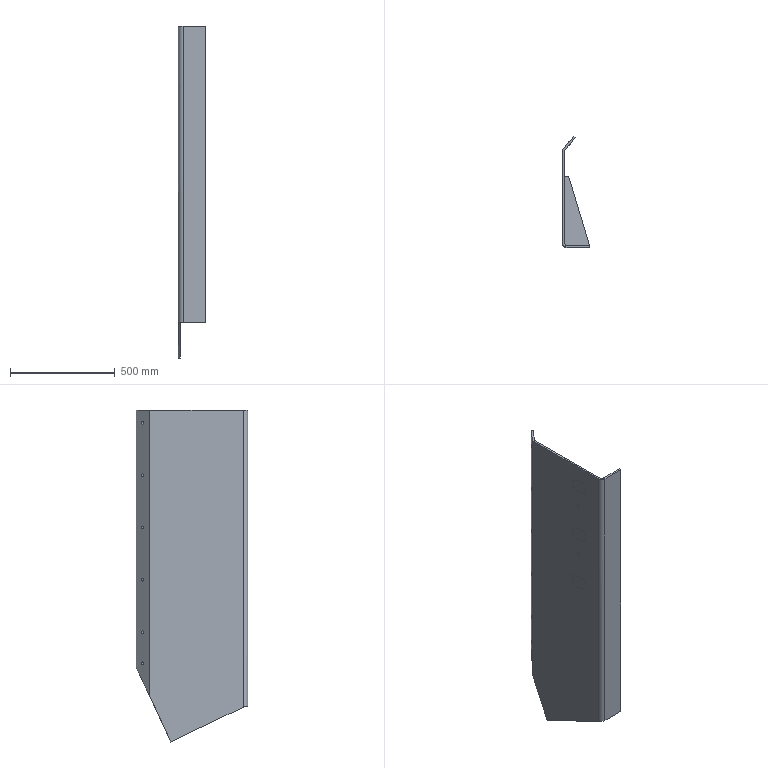Part | STEP file | Edge plate 2_Default<As machined> | 5 solids | 78 faces | box 130 x 532.359 x 1587 mm | volume 10246266 mm3 | plane 53 | cylinder 25 | commonest cylinder face diameters 14 x12 24 x5 17 x4 30 x3 44 x1